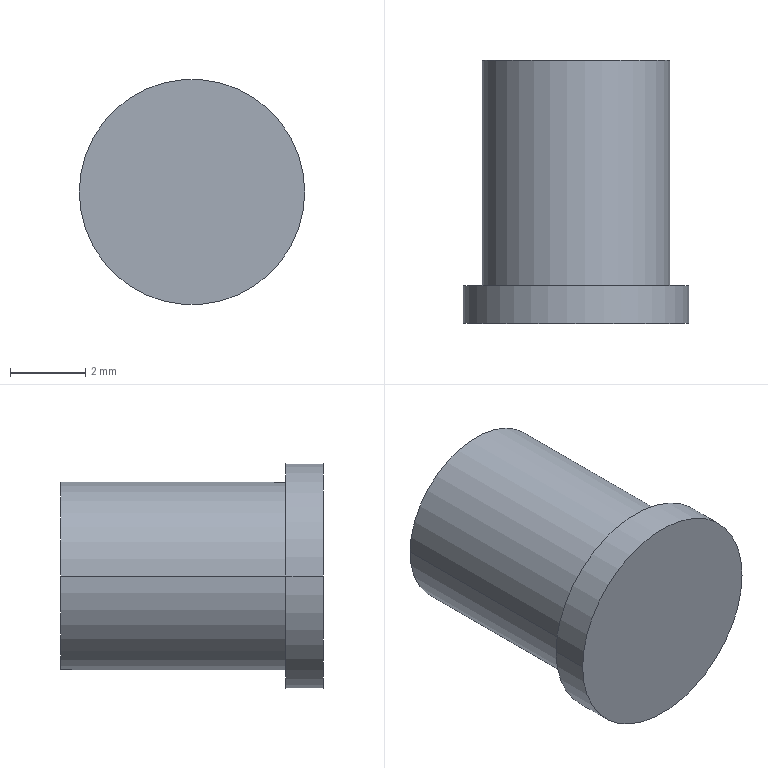Part | STEP file | JDC-75-4 | 1 solid | 7 faces | box 6 x 7 x 6 mm | volume 146.084 mm3 | cylinder 4 | plane 3 | commonest cylinder face diameters 5 x2 6 x2
STEP:
#1=CARTESIAN_POINT('',(0.,0.,0.));
#2=DIRECTION('',(0.,0.,1.));
#3=DIRECTION('',(1.,0.,0.));
#4=AXIS2_PLACEMENT_3D('',#1,#2,#3);
#5=CARTESIAN_POINT('',(-2.5,7.,0.));
#6=VERTEX_POINT('',#5);
#7=CARTESIAN_POINT('',(2.5,7.,0.));
#8=VERTEX_POINT('',#7);
#9=CARTESIAN_POINT('',(0.,7.,0.));
#10=DIRECTION('',(0.,1.,0.));
#11=DIRECTION('',(-1.,0.,0.));
#12=AXIS2_PLACEMENT_3D('',#9,#10,#11);
#13=CIRCLE('',#12,2.5);
#14=CARTESIAN_POINT('',(2.5,7.,0.));
#15=DIRECTION('',(0.,1.,0.));
#16=DIRECTION('',(-1.,0.,0.));
#17=AXIS2_PLACEMENT_3D('',#14,#15,#16);
#18=PLANE('',#17);
#19=CARTESIAN_POINT('',(2.5,0.));
#20=DIRECTION('',(1.,0.));
#21=AXIS2_PLACEMENT_2D('',#19,#20);
#22=CIRCLE('',#21,2.5);
#23=(GEOMETRIC_REPRESENTATION_CONTEXT(2)PARAMETRIC_REPRESENTATION_CONTEXT()REPRESENTATION_CONTEXT('',''));
#24=DEFINITIONAL_REPRESENTATION('',(#22),#23);
#25=PCURVE('',#18,#24);
#26=CARTESIAN_POINT('',(0.,-240.9,0.));
#27=DIRECTION('',(0.,-1.,0.));
#28=DIRECTION('',(1.,0.,0.));
#29=AXIS2_PLACEMENT_3D('',#26,#27,#28);
#30=CYLINDRICAL_SURFACE('',#29,2.5);
#31=CARTESIAN_POINT('',(3.142,-247.9));
#32=DIRECTION('',(-1.,0.));
#33=VECTOR('',#32,1.);
#34=LINE('',#31,#33);
#35=(GEOMETRIC_REPRESENTATION_CONTEXT(2)PARAMETRIC_REPRESENTATION_CONTEXT()REPRESENTATION_CONTEXT('',''));
#36=DEFINITIONAL_REPRESENTATION('',(#34),#35);
#37=PCURVE('',#30,#36);
#38=SURFACE_CURVE('',#13,(#25,#37),.PCURVE_S1.);
#39=EDGE_CURVE('',#6,#8,#38,.T.);
#40=ORIENTED_EDGE('',*,*,#39,.F.);
#41=CARTESIAN_POINT('',(0.,7.,0.));
#42=DIRECTION('',(0.,1.,0.));
#43=DIRECTION('',(1.,0.,0.));
#44=AXIS2_PLACEMENT_3D('',#41,#42,#43);
#45=CIRCLE('',#44,2.5);
#46=CARTESIAN_POINT('',(2.5,0.));
#47=DIRECTION('',(-1.,0.));
#48=AXIS2_PLACEMENT_2D('',#46,#47);
#49=CIRCLE('',#48,2.5);
#50=(GEOMETRIC_REPRESENTATION_CONTEXT(2)PARAMETRIC_REPRESENTATION_CONTEXT()REPRESENTATION_CONTEXT('',''));
#51=DEFINITIONAL_REPRESENTATION('',(#49),#50);
#52=PCURVE('',#18,#51);
#53=CARTESIAN_POINT('',(0.,-240.9,0.));
#54=DIRECTION('',(0.,-1.,0.));
#55=DIRECTION('',(1.,0.,0.));
#56=AXIS2_PLACEMENT_3D('',#53,#54,#55);
#57=CYLINDRICAL_SURFACE('',#56,2.5);
#58=CARTESIAN_POINT('',(6.283,-247.9));
#59=DIRECTION('',(-1.,0.));
#60=VECTOR('',#59,1.);
#61=LINE('',#58,#60);
#62=(GEOMETRIC_REPRESENTATION_CONTEXT(2)PARAMETRIC_REPRESENTATION_CONTEXT()REPRESENTATION_CONTEXT('',''));
#63=DEFINITIONAL_REPRESENTATION('',(#61),#62);
#64=PCURVE('',#57,#63);
#65=SURFACE_CURVE('',#45,(#52,#64),.PCURVE_S1.);
#66=EDGE_CURVE('',#8,#6,#65,.T.);
#67=ORIENTED_EDGE('',*,*,#66,.F.);
#68=EDGE_LOOP('',(#40,#67));
#69=FACE_BOUND('',#68,.F.);
#70=ADVANCED_FACE('',(#69),#18,.T.);
#71=CARTESIAN_POINT('',(-2.5,1.,0.));
#72=VERTEX_POINT('',#71);
#73=CARTESIAN_POINT('',(-2.5,1.,0.));
#74=DIRECTION('',(0.,1.,0.));
#75=VECTOR('',#74,1.);
#76=LINE('',#73,#75);
#77=CARTESIAN_POINT('',(3.142,-241.9));
#78=DIRECTION('',(0.,-1.));
#79=VECTOR('',#78,1.);
#80=LINE('',#77,#79);
#81=(GEOMETRIC_REPRESENTATION_CONTEXT(2)PARAMETRIC_REPRESENTATION_CONTEXT()REPRESENTATION_CONTEXT('',''));
#82=DEFINITIONAL_REPRESENTATION('',(#80),#81);
#83=PCURVE('',#30,#82);
#84=CARTESIAN_POINT('',(3.142,-241.9));
#85=DIRECTION('',(0.,-1.));
#86=VECTOR('',#85,1.);
#87=LINE('',#84,#86);
#88=(GEOMETRIC_REPRESENTATION_CONTEXT(2)PARAMETRIC_REPRESENTATION_CONTEXT()REPRESENTATION_CONTEXT('',''));
#89=DEFINITIONAL_REPRESENTATION('',(#87),#88);
#90=PCURVE('',#57,#89);
#91=SURFACE_CURVE('',#76,(#83,#90),.PCURVE_S1.);
#92=EDGE_CURVE('',#72,#6,#91,.T.);
#93=ORIENTED_EDGE('',*,*,#92,.F.);
#94=CARTESIAN_POINT('',(2.5,1.,0.));
#95=VERTEX_POINT('',#94);
#96=CARTESIAN_POINT('',(0.,1.,0.));
#97=DIRECTION('',(0.,-1.,0.));
#98=DIRECTION('',(1.,0.,0.));
#99=AXIS2_PLACEMENT_3D('',#96,#97,#98);
#100=CIRCLE('',#99,2.5);
#101=CARTESIAN_POINT('',(0.,-241.9));
#102=DIRECTION('',(1.,0.));
#103=VECTOR('',#102,1.);
#104=LINE('',#101,#103);
#105=(GEOMETRIC_REPRESENTATION_CONTEXT(2)PARAMETRIC_REPRESENTATION_CONTEXT()REPRESENTATION_CONTEXT('',''));
#106=DEFINITIONAL_REPRESENTATION('',(#104),#105);
#107=PCURVE('',#30,#106);
#108=CARTESIAN_POINT('',(3.,1.,0.));
#109=DIRECTION('',(0.,1.,0.));
#110=DIRECTION('',(-1.,0.,0.));
#111=AXIS2_PLACEMENT_3D('',#108,#109,#110);
#112=PLANE('',#111);
#113=CARTESIAN_POINT('',(0.5,0.));
#114=CARTESIAN_POINT('',(0.5,4.33));
#115=CARTESIAN_POINT('',(4.25,2.165));
#116=CARTESIAN_POINT('',(8.,0.));
#117=CARTESIAN_POINT('',(4.25,-2.165));
#118=CARTESIAN_POINT('',(0.5,-4.33));
#119=CARTESIAN_POINT('',(0.5,0.));
#120=(BOUNDED_CURVE()B_SPLINE_CURVE(2,(#113,#114,#115,#116,#117,#118,#119),.UNSPECIFIED.,.T.,.F.)B_SPLINE_CURVE_WITH_KNOTS((1,2,2,2,2,1),(-2.094,0.,2.094,4.189,6.283,8.378),.UNSPECIFIED.)CURVE()GEOMETRIC_REPRESENTATION_ITEM()RATIONAL_B_SPLINE_CURVE((1.,0.5,1.,0.5,1.,0.5,1.))REPRESENTATION_ITEM(''));
#121=(GEOMETRIC_REPRESENTATION_CONTEXT(2)PARAMETRIC_REPRESENTATION_CONTEXT()REPRESENTATION_CONTEXT('',''));
#122=DEFINITIONAL_REPRESENTATION('',(#120),#121);
#123=PCURVE('',#112,#122);
#124=SURFACE_CURVE('',#100,(#107,#123),.PCURVE_S1.);
#125=EDGE_CURVE('',#95,#72,#124,.T.);
#126=ORIENTED_EDGE('',*,*,#125,.F.);
#127=CARTESIAN_POINT('',(2.5,1.,0.));
#128=DIRECTION('',(0.,1.,0.));
#129=VECTOR('',#128,1.);
#130=LINE('',#127,#129);
#131=CARTESIAN_POINT('',(0.,-241.9));
#132=DIRECTION('',(0.,-1.));
#133=VECTOR('',#132,1.);
#134=LINE('',#131,#133);
#135=(GEOMETRIC_REPRESENTATION_CONTEXT(2)PARAMETRIC_REPRESENTATION_CONTEXT()REPRESENTATION_CONTEXT('',''));
#136=DEFINITIONAL_REPRESENTATION('',(#134),#135);
#137=PCURVE('',#30,#136);
#138=CARTESIAN_POINT('',(6.283,-241.9));
#139=DIRECTION('',(0.,-1.));
#140=VECTOR('',#139,1.);
#141=LINE('',#138,#140);
#142=(GEOMETRIC_REPRESENTATION_CONTEXT(2)PARAMETRIC_REPRESENTATION_CONTEXT()REPRESENTATION_CONTEXT('',''));
#143=DEFINITIONAL_REPRESENTATION('',(#141),#142);
#144=PCURVE('',#57,#143);
#145=SURFACE_CURVE('',#130,(#137,#144),.PCURVE_S1.);
#146=EDGE_CURVE('',#95,#8,#145,.T.);
#147=ORIENTED_EDGE('',*,*,#146,.T.);
#148=ORIENTED_EDGE('',*,*,#39,.F.);
#149=EDGE_LOOP('',(#93,#126,#147,#148));
#150=FACE_BOUND('',#149,.T.);
#151=ADVANCED_FACE('',(#150),#30,.T.);
#152=ORIENTED_EDGE('',*,*,#66,.F.);
#153=ORIENTED_EDGE('',*,*,#146,.F.);
#154=CARTESIAN_POINT('',(0.,1.,0.));
#155=DIRECTION('',(0.,-1.,0.));
#156=DIRECTION('',(-1.,0.,0.));
#157=AXIS2_PLACEMENT_3D('',#154,#155,#156);
#158=CIRCLE('',#157,2.5);
#159=CARTESIAN_POINT('',(3.142,-241.9));
#160=DIRECTION('',(1.,0.));
#161=VECTOR('',#160,1.);
#162=LINE('',#159,#161);
#163=(GEOMETRIC_REPRESENTATION_CONTEXT(2)PARAMETRIC_REPRESENTATION_CONTEXT()REPRESENTATION_CONTEXT('',''));
#164=DEFINITIONAL_REPRESENTATION('',(#162),#163);
#165=PCURVE('',#57,#164);
#166=CARTESIAN_POINT('',(5.5,0.));
#167=CARTESIAN_POINT('',(5.5,-4.33));
#168=CARTESIAN_POINT('',(1.75,-2.165));
#169=CARTESIAN_POINT('',(-2.,0.));
#170=CARTESIAN_POINT('',(1.75,2.165));
#171=CARTESIAN_POINT('',(5.5,4.33));
#172=CARTESIAN_POINT('',(5.5,0.));
#173=(BOUNDED_CURVE()B_SPLINE_CURVE(2,(#166,#167,#168,#169,#170,#171,#172),.UNSPECIFIED.,.T.,.F.)B_SPLINE_CURVE_WITH_KNOTS((1,2,2,2,2,1),(-2.094,0.,2.094,4.189,6.283,8.378),.UNSPECIFIED.)CURVE()GEOMETRIC_REPRESENTATION_ITEM()RATIONAL_B_SPLINE_CURVE((1.,0.5,1.,0.5,1.,0.5,1.))REPRESENTATION_ITEM(''));
#174=(GEOMETRIC_REPRESENTATION_CONTEXT(2)PARAMETRIC_REPRESENTATION_CONTEXT()REPRESENTATION_CONTEXT('',''));
#175=DEFINITIONAL_REPRESENTATION('',(#173),#174);
#176=PCURVE('',#112,#175);
#177=SURFACE_CURVE('',#158,(#165,#176),.PCURVE_S1.);
#178=EDGE_CURVE('',#72,#95,#177,.T.);
#179=ORIENTED_EDGE('',*,*,#178,.F.);
#180=ORIENTED_EDGE('',*,*,#92,.T.);
#181=EDGE_LOOP('',(#152,#153,#179,#180));
#182=FACE_BOUND('',#181,.T.);
#183=ADVANCED_FACE('',(#182),#57,.T.);
#184=CARTESIAN_POINT('',(-3.,1.,0.));
#185=VERTEX_POINT('',#184);
#186=CARTESIAN_POINT('',(3.,1.,0.));
#187=VERTEX_POINT('',#186);
#188=CARTESIAN_POINT('',(0.,1.,0.));
#189=DIRECTION('',(0.,1.,0.));
#190=DIRECTION('',(-1.,0.,0.));
#191=AXIS2_PLACEMENT_3D('',#188,#189,#190);
#192=CIRCLE('',#191,3.);
#193=CARTESIAN_POINT('',(3.,0.));
#194=DIRECTION('',(1.,0.));
#195=AXIS2_PLACEMENT_2D('',#193,#194);
#196=CIRCLE('',#195,3.);
#197=(GEOMETRIC_REPRESENTATION_CONTEXT(2)PARAMETRIC_REPRESENTATION_CONTEXT()REPRESENTATION_CONTEXT('',''));
#198=DEFINITIONAL_REPRESENTATION('',(#196),#197);
#199=PCURVE('',#112,#198);
#200=CARTESIAN_POINT('',(0.,-240.9,0.));
#201=DIRECTION('',(0.,-1.,0.));
#202=DIRECTION('',(1.,0.,0.));
#203=AXIS2_PLACEMENT_3D('',#200,#201,#202);
#204=CYLINDRICAL_SURFACE('',#203,3.);
#205=CARTESIAN_POINT('',(3.142,-241.9));
#206=DIRECTION('',(-1.,0.));
#207=VECTOR('',#206,1.);
#208=LINE('',#205,#207);
#209=(GEOMETRIC_REPRESENTATION_CONTEXT(2)PARAMETRIC_REPRESENTATION_CONTEXT()REPRESENTATION_CONTEXT('',''));
#210=DEFINITIONAL_REPRESENTATION('',(#208),#209);
#211=PCURVE('',#204,#210);
#212=SURFACE_CURVE('',#192,(#199,#211),.PCURVE_S1.);
#213=EDGE_CURVE('',#185,#187,#212,.T.);
#214=ORIENTED_EDGE('',*,*,#213,.F.);
#215=CARTESIAN_POINT('',(0.,1.,0.));
#216=DIRECTION('',(0.,1.,0.));
#217=DIRECTION('',(1.,0.,0.));
#218=AXIS2_PLACEMENT_3D('',#215,#216,#217);
#219=CIRCLE('',#218,3.);
#220=CARTESIAN_POINT('',(3.,0.));
#221=DIRECTION('',(-1.,0.));
#222=AXIS2_PLACEMENT_2D('',#220,#221);
#223=CIRCLE('',#222,3.);
#224=(GEOMETRIC_REPRESENTATION_CONTEXT(2)PARAMETRIC_REPRESENTATION_CONTEXT()REPRESENTATION_CONTEXT('',''));
#225=DEFINITIONAL_REPRESENTATION('',(#223),#224);
#226=PCURVE('',#112,#225);
#227=CARTESIAN_POINT('',(0.,-240.9,0.));
#228=DIRECTION('',(0.,-1.,0.));
#229=DIRECTION('',(1.,0.,0.));
#230=AXIS2_PLACEMENT_3D('',#227,#228,#229);
#231=CYLINDRICAL_SURFACE('',#230,3.);
#232=CARTESIAN_POINT('',(6.283,-241.9));
#233=DIRECTION('',(-1.,0.));
#234=VECTOR('',#233,1.);
#235=LINE('',#232,#234);
#236=(GEOMETRIC_REPRESENTATION_CONTEXT(2)PARAMETRIC_REPRESENTATION_CONTEXT()REPRESENTATION_CONTEXT('',''));
#237=DEFINITIONAL_REPRESENTATION('',(#235),#236);
#238=PCURVE('',#231,#237);
#239=SURFACE_CURVE('',#219,(#226,#238),.PCURVE_S1.);
#240=EDGE_CURVE('',#187,#185,#239,.T.);
#241=ORIENTED_EDGE('',*,*,#240,.F.);
#242=EDGE_LOOP('',(#214,#241));
#243=FACE_BOUND('',#242,.F.);
#244=ORIENTED_EDGE('',*,*,#125,.F.);
#245=ORIENTED_EDGE('',*,*,#178,.F.);
#246=EDGE_LOOP('',(#244,#245));
#247=FACE_BOUND('',#246,.F.);
#248=ADVANCED_FACE('',(#243,#247),#112,.T.);
#249=CARTESIAN_POINT('',(-3.,0.,0.));
#250=VERTEX_POINT('',#249);
#251=CARTESIAN_POINT('',(-3.,0.,0.));
#252=DIRECTION('',(0.,1.,0.));
#253=VECTOR('',#252,1.);
#254=LINE('',#251,#253);
#255=CARTESIAN_POINT('',(3.142,-240.9));
#256=DIRECTION('',(0.,-1.));
#257=VECTOR('',#256,1.);
#258=LINE('',#255,#257);
#259=(GEOMETRIC_REPRESENTATION_CONTEXT(2)PARAMETRIC_REPRESENTATION_CONTEXT()REPRESENTATION_CONTEXT('',''));
#260=DEFINITIONAL_REPRESENTATION('',(#258),#259);
#261=PCURVE('',#204,#260);
#262=CARTESIAN_POINT('',(3.142,-240.9));
#263=DIRECTION('',(0.,-1.));
#264=VECTOR('',#263,1.);
#265=LINE('',#262,#264);
#266=(GEOMETRIC_REPRESENTATION_CONTEXT(2)PARAMETRIC_REPRESENTATION_CONTEXT()REPRESENTATION_CONTEXT('',''));
#267=DEFINITIONAL_REPRESENTATION('',(#265),#266);
#268=PCURVE('',#231,#267);
#269=SURFACE_CURVE('',#254,(#261,#268),.PCURVE_S1.);
#270=EDGE_CURVE('',#250,#185,#269,.T.);
#271=ORIENTED_EDGE('',*,*,#270,.F.);
#272=CARTESIAN_POINT('',(3.,0.,0.));
#273=VERTEX_POINT('',#272);
#274=CARTESIAN_POINT('',(0.,0.,0.));
#275=DIRECTION('',(0.,-1.,0.));
#276=DIRECTION('',(1.,0.,0.));
#277=AXIS2_PLACEMENT_3D('',#274,#275,#276);
#278=CIRCLE('',#277,3.);
#279=CARTESIAN_POINT('',(0.,-240.9));
#280=DIRECTION('',(1.,0.));
#281=VECTOR('',#280,1.);
#282=LINE('',#279,#281);
#283=(GEOMETRIC_REPRESENTATION_CONTEXT(2)PARAMETRIC_REPRESENTATION_CONTEXT()REPRESENTATION_CONTEXT('',''));
#284=DEFINITIONAL_REPRESENTATION('',(#282),#283);
#285=PCURVE('',#204,#284);
#286=CARTESIAN_POINT('',(0.,0.,0.));
#287=DIRECTION('',(0.,-1.,0.));
#288=DIRECTION('',(1.,0.,0.));
#289=AXIS2_PLACEMENT_3D('',#286,#287,#288);
#290=PLANE('',#289);
#291=CARTESIAN_POINT('',(0.,0.));
#292=DIRECTION('',(1.,0.));
#293=AXIS2_PLACEMENT_2D('',#291,#292);
#294=CIRCLE('',#293,3.);
#295=(GEOMETRIC_REPRESENTATION_CONTEXT(2)PARAMETRIC_REPRESENTATION_CONTEXT()REPRESENTATION_CONTEXT('',''));
#296=DEFINITIONAL_REPRESENTATION('',(#294),#295);
#297=PCURVE('',#290,#296);
#298=SURFACE_CURVE('',#278,(#285,#297),.PCURVE_S1.);
#299=EDGE_CURVE('',#273,#250,#298,.T.);
#300=ORIENTED_EDGE('',*,*,#299,.F.);
#301=CARTESIAN_POINT('',(3.,0.,0.));
#302=DIRECTION('',(0.,1.,0.));
#303=VECTOR('',#302,1.);
#304=LINE('',#301,#303);
#305=CARTESIAN_POINT('',(0.,-240.9));
#306=DIRECTION('',(0.,-1.));
#307=VECTOR('',#306,1.);
#308=LINE('',#305,#307);
#309=(GEOMETRIC_REPRESENTATION_CONTEXT(2)PARAMETRIC_REPRESENTATION_CONTEXT()REPRESENTATION_CONTEXT('',''));
#310=DEFINITIONAL_REPRESENTATION('',(#308),#309);
#311=PCURVE('',#204,#310);
#312=CARTESIAN_POINT('',(6.283,-240.9));
#313=DIRECTION('',(0.,-1.));
#314=VECTOR('',#313,1.);
#315=LINE('',#312,#314);
#316=(GEOMETRIC_REPRESENTATION_CONTEXT(2)PARAMETRIC_REPRESENTATION_CONTEXT()REPRESENTATION_CONTEXT('',''));
#317=DEFINITIONAL_REPRESENTATION('',(#315),#316);
#318=PCURVE('',#231,#317);
#319=SURFACE_CURVE('',#304,(#311,#318),.PCURVE_S1.);
#320=EDGE_CURVE('',#273,#187,#319,.T.);
#321=ORIENTED_EDGE('',*,*,#320,.T.);
#322=ORIENTED_EDGE('',*,*,#213,.F.);
#323=EDGE_LOOP('',(#271,#300,#321,#322));
#324=FACE_BOUND('',#323,.T.);
#325=ADVANCED_FACE('',(#324),#204,.T.);
#326=ORIENTED_EDGE('',*,*,#240,.F.);
#327=ORIENTED_EDGE('',*,*,#320,.F.);
#328=CARTESIAN_POINT('',(0.,0.,0.));
#329=DIRECTION('',(0.,-1.,0.));
#330=DIRECTION('',(-1.,0.,0.));
#331=AXIS2_PLACEMENT_3D('',#328,#329,#330);
#332=CIRCLE('',#331,3.);
#333=CARTESIAN_POINT('',(3.142,-240.9));
#334=DIRECTION('',(1.,0.));
#335=VECTOR('',#334,1.);
#336=LINE('',#333,#335);
#337=(GEOMETRIC_REPRESENTATION_CONTEXT(2)PARAMETRIC_REPRESENTATION_CONTEXT()REPRESENTATION_CONTEXT('',''));
#338=DEFINITIONAL_REPRESENTATION('',(#336),#337);
#339=PCURVE('',#231,#338);
#340=CARTESIAN_POINT('',(0.,0.));
#341=DIRECTION('',(-1.,0.));
#342=AXIS2_PLACEMENT_2D('',#340,#341);
#343=CIRCLE('',#342,3.);
#344=(GEOMETRIC_REPRESENTATION_CONTEXT(2)PARAMETRIC_REPRESENTATION_CONTEXT()REPRESENTATION_CONTEXT('',''));
#345=DEFINITIONAL_REPRESENTATION('',(#343),#344);
#346=PCURVE('',#290,#345);
#347=SURFACE_CURVE('',#332,(#339,#346),.PCURVE_S1.);
#348=EDGE_CURVE('',#250,#273,#347,.T.);
#349=ORIENTED_EDGE('',*,*,#348,.F.);
#350=ORIENTED_EDGE('',*,*,#270,.T.);
#351=EDGE_LOOP('',(#326,#327,#349,#350));
#352=FACE_BOUND('',#351,.T.);
#353=ADVANCED_FACE('',(#352),#231,.T.);
#354=ORIENTED_EDGE('',*,*,#299,.F.);
#355=ORIENTED_EDGE('',*,*,#348,.F.);
#356=EDGE_LOOP('',(#354,#355));
#357=FACE_BOUND('',#356,.F.);
#358=ADVANCED_FACE('',(#357),#290,.T.);
#359=CLOSED_SHELL('',(#70,#151,#183,#248,#325,#353,#358));
#360=MANIFOLD_SOLID_BREP('',#359);
#361=(LENGTH_UNIT()NAMED_UNIT(*)SI_UNIT(.MILLI.,.METRE.));
#362=UNCERTAINTY_MEASURE_WITH_UNIT(LENGTH_MEASURE(0.0000001),#361,'','');
#363=(NAMED_UNIT(*)PLANE_ANGLE_UNIT()SI_UNIT($,.RADIAN.));
#364=(NAMED_UNIT(*)SI_UNIT($,.STERADIAN.)SOLID_ANGLE_UNIT());
#365=(GEOMETRIC_REPRESENTATION_CONTEXT(3)GLOBAL_UNCERTAINTY_ASSIGNED_CONTEXT((#362))GLOBAL_UNIT_ASSIGNED_CONTEXT((#361,#363,#364))REPRESENTATION_CONTEXT('',''));
#366=ADVANCED_BREP_SHAPE_REPRESENTATION('',(#4,#360),#365);